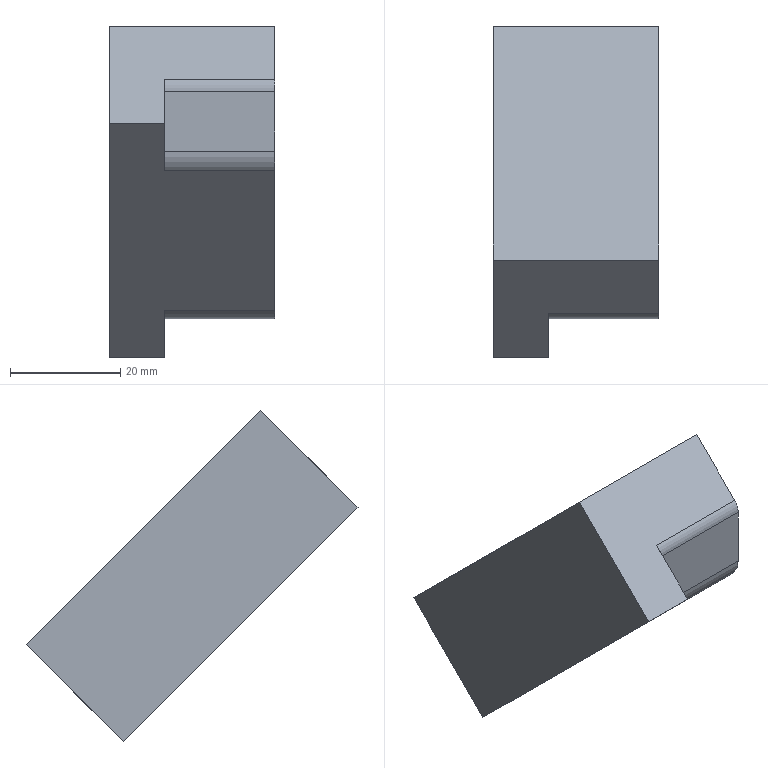Part | NX | features solid 2 | 1 solid | 14 faces | box 30 x 60.104 x 60.104 mm | volume 42971 mm3 | plane 10 | cylinder 4 | commonest cylinder face diameters 6 x2 10 x2
STEP:
#1=CARTESIAN_POINT('',(735.,899.35,-213.579));
#2=VERTEX_POINT('',#1);
#3=CARTESIAN_POINT('',(735.,907.3,-205.629));
#4=VERTEX_POINT('',#3);
#5=CARTESIAN_POINT('',(735.,899.35,-213.579));
#6=DIRECTION('',(0.,0.7071,0.7071));
#7=VECTOR('',#6,1000.);
#8=LINE('',#5,#7);
#9=EDGE_CURVE('',#2,#4,#8,.T.);
#10=ORIENTED_EDGE('',*,*,#9,.F.);
#11=CARTESIAN_POINT('',(735.,907.886,-222.114));
#12=VERTEX_POINT('',#11);
#13=CARTESIAN_POINT('',(735.,899.35,-213.579));
#14=DIRECTION('',(0.,0.7071,-0.7071));
#15=VECTOR('',#14,1000.);
#16=LINE('',#13,#15);
#17=EDGE_CURVE('',#2,#12,#16,.T.);
#18=ORIENTED_EDGE('',*,*,#17,.T.);
#19=CARTESIAN_POINT('',(735.,906.421,-218.579));
#20=VERTEX_POINT('',#19);
#21=CARTESIAN_POINT('',(735.,911.421,-218.579));
#22=DIRECTION('',(-1.,0.,0.));
#23=DIRECTION('',(0.,0.9962,0.08716));
#24=AXIS2_PLACEMENT_3D('',#21,#22,#23);
#25=CIRCLE('',#24,5.);
#26=EDGE_CURVE('',#20,#12,#25,.F.);
#27=ORIENTED_EDGE('',*,*,#26,.F.);
#28=CARTESIAN_POINT('',(735.,906.421,-207.75));
#29=VERTEX_POINT('',#28);
#30=CARTESIAN_POINT('',(735.,906.421,-256.005));
#31=DIRECTION('',(0.,0.,-1.));
#32=VECTOR('',#31,1000.);
#33=LINE('',#30,#32);
#34=EDGE_CURVE('',#29,#20,#33,.T.);
#35=ORIENTED_EDGE('',*,*,#34,.F.);
#36=CARTESIAN_POINT('',(735.,909.421,-207.75));
#37=DIRECTION('',(-1.,0.,0.));
#38=DIRECTION('',(0.,0.9962,0.08716));
#39=AXIS2_PLACEMENT_3D('',#36,#37,#38);
#40=CIRCLE('',#39,3.);
#41=EDGE_CURVE('',#4,#29,#40,.F.);
#42=ORIENTED_EDGE('',*,*,#41,.F.);
#43=EDGE_LOOP('',(#10,#18,#27,#35,#42));
#44=FACE_BOUND('',#43,.T.);
#45=CARTESIAN_POINT('',(735.,941.777,-256.005));
#46=DIRECTION('',(1.,0.,0.));
#47=DIRECTION('',(0.,0.9962,0.08716));
#48=AXIS2_PLACEMENT_3D('',#45,#46,#47);
#49=PLANE('',#48);
#50=ADVANCED_FACE('',(#44),#49,.T.);
#51=CARTESIAN_POINT('',(735.,933.241,-247.47));
#52=VERTEX_POINT('',#51);
#53=CARTESIAN_POINT('',(735.,941.777,-256.005));
#54=VERTEX_POINT('',#53);
#55=CARTESIAN_POINT('',(735.,899.35,-213.579));
#56=DIRECTION('',(0.,0.7071,-0.7071));
#57=VECTOR('',#56,1000.);
#58=LINE('',#55,#57);
#59=EDGE_CURVE('',#52,#54,#58,.T.);
#60=ORIENTED_EDGE('',*,*,#59,.T.);
#61=CARTESIAN_POINT('',(735.,949.726,-248.055));
#62=VERTEX_POINT('',#61);
#63=CARTESIAN_POINT('',(735.,941.777,-256.005));
#64=DIRECTION('',(0.,0.7071,0.7071));
#65=VECTOR('',#64,1000.);
#66=LINE('',#63,#65);
#67=EDGE_CURVE('',#54,#62,#66,.T.);
#68=ORIENTED_EDGE('',*,*,#67,.T.);
#69=CARTESIAN_POINT('',(735.,947.605,-248.934));
#70=VERTEX_POINT('',#69);
#71=CARTESIAN_POINT('',(735.,947.605,-245.934));
#72=DIRECTION('',(-1.,0.,0.));
#73=DIRECTION('',(0.,0.9962,0.08716));
#74=AXIS2_PLACEMENT_3D('',#71,#72,#73);
#75=CIRCLE('',#74,3.);
#76=EDGE_CURVE('',#70,#62,#75,.F.);
#77=ORIENTED_EDGE('',*,*,#76,.F.);
#78=CARTESIAN_POINT('',(735.,936.777,-248.934));
#79=VERTEX_POINT('',#78);
#80=CARTESIAN_POINT('',(735.,941.777,-248.934));
#81=DIRECTION('',(0.,1.,0.));
#82=VECTOR('',#81,1000.);
#83=LINE('',#80,#82);
#84=EDGE_CURVE('',#79,#70,#83,.T.);
#85=ORIENTED_EDGE('',*,*,#84,.F.);
#86=CARTESIAN_POINT('',(735.,936.777,-243.934));
#87=DIRECTION('',(-1.,0.,0.));
#88=DIRECTION('',(0.,0.9962,0.08716));
#89=AXIS2_PLACEMENT_3D('',#86,#87,#88);
#90=CIRCLE('',#89,5.);
#91=EDGE_CURVE('',#52,#79,#90,.F.);
#92=ORIENTED_EDGE('',*,*,#91,.F.);
#93=EDGE_LOOP('',(#60,#68,#77,#85,#92));
#94=FACE_BOUND('',#93,.T.);
#95=CARTESIAN_POINT('',(735.,941.777,-256.005));
#96=DIRECTION('',(1.,0.,0.));
#97=DIRECTION('',(0.,0.9962,0.08716));
#98=AXIS2_PLACEMENT_3D('',#95,#96,#97);
#99=PLANE('',#98);
#100=ADVANCED_FACE('',(#94),#99,.T.);
#101=ORIENTED_EDGE('',*,*,#67,.F.);
#102=CARTESIAN_POINT('',(725.,941.777,-256.005));
#103=VERTEX_POINT('',#102);
#104=CARTESIAN_POINT('',(735.,941.777,-256.005));
#105=DIRECTION('',(-1.,0.,0.));
#106=VECTOR('',#105,1000.);
#107=LINE('',#104,#106);
#108=EDGE_CURVE('',#54,#103,#107,.T.);
#109=ORIENTED_EDGE('',*,*,#108,.T.);
#110=CARTESIAN_POINT('',(725.,959.454,-238.327));
#111=VERTEX_POINT('',#110);
#112=CARTESIAN_POINT('',(725.,941.777,-256.005));
#113=DIRECTION('',(0.,0.7071,0.7071));
#114=VECTOR('',#113,1000.);
#115=LINE('',#112,#114);
#116=EDGE_CURVE('',#103,#111,#115,.T.);
#117=ORIENTED_EDGE('',*,*,#116,.T.);
#118=CARTESIAN_POINT('',(755.,959.454,-238.327));
#119=VERTEX_POINT('',#118);
#120=CARTESIAN_POINT('',(735.,959.454,-238.327));
#121=DIRECTION('',(-1.,0.,0.));
#122=VECTOR('',#121,1000.);
#123=LINE('',#120,#122);
#124=EDGE_CURVE('',#119,#111,#123,.T.);
#125=ORIENTED_EDGE('',*,*,#124,.F.);
#126=CARTESIAN_POINT('',(755.,949.726,-248.055));
#127=VERTEX_POINT('',#126);
#128=CARTESIAN_POINT('',(755.,941.777,-256.005));
#129=DIRECTION('',(0.,0.7071,0.7071));
#130=VECTOR('',#129,1000.);
#131=LINE('',#128,#130);
#132=EDGE_CURVE('',#127,#119,#131,.T.);
#133=ORIENTED_EDGE('',*,*,#132,.F.);
#134=CARTESIAN_POINT('',(755.,949.726,-248.055));
#135=DIRECTION('',(-1.,0.,0.));
#136=VECTOR('',#135,1000.);
#137=LINE('',#134,#136);
#138=EDGE_CURVE('',#62,#127,#137,.F.);
#139=ORIENTED_EDGE('',*,*,#138,.F.);
#140=EDGE_LOOP('',(#101,#109,#117,#125,#133,#139));
#141=FACE_BOUND('',#140,.T.);
#142=CARTESIAN_POINT('',(735.,941.777,-256.005));
#143=DIRECTION('',(0.,0.7071,-0.7071));
#144=DIRECTION('',(0.,0.7071,0.7071));
#145=AXIS2_PLACEMENT_3D('',#142,#143,#144);
#146=PLANE('',#145);
#147=ADVANCED_FACE('',(#141),#146,.T.);
#148=CARTESIAN_POINT('',(725.,917.028,-195.901));
#149=VERTEX_POINT('',#148);
#150=CARTESIAN_POINT('',(725.,917.028,-195.901));
#151=DIRECTION('',(0.,0.7071,-0.7071));
#152=VECTOR('',#151,1000.);
#153=LINE('',#150,#152);
#154=EDGE_CURVE('',#149,#111,#153,.T.);
#155=ORIENTED_EDGE('',*,*,#154,.F.);
#156=CARTESIAN_POINT('',(755.,917.028,-195.901));
#157=VERTEX_POINT('',#156);
#158=CARTESIAN_POINT('',(735.,917.028,-195.901));
#159=DIRECTION('',(-1.,0.,0.));
#160=VECTOR('',#159,1000.);
#161=LINE('',#158,#160);
#162=EDGE_CURVE('',#157,#149,#161,.T.);
#163=ORIENTED_EDGE('',*,*,#162,.F.);
#164=CARTESIAN_POINT('',(755.,917.028,-195.901));
#165=DIRECTION('',(0.,0.7071,-0.7071));
#166=VECTOR('',#165,1000.);
#167=LINE('',#164,#166);
#168=EDGE_CURVE('',#157,#119,#167,.T.);
#169=ORIENTED_EDGE('',*,*,#168,.T.);
#170=ORIENTED_EDGE('',*,*,#124,.T.);
#171=EDGE_LOOP('',(#155,#163,#169,#170));
#172=FACE_BOUND('',#171,.T.);
#173=CARTESIAN_POINT('',(735.,917.028,-195.901));
#174=DIRECTION('',(0.,-0.7071,-0.7071));
#175=DIRECTION('',(0.,0.7071,-0.7071));
#176=AXIS2_PLACEMENT_3D('',#173,#174,#175);
#177=PLANE('',#176);
#178=ADVANCED_FACE('',(#172),#177,.F.);
#179=CARTESIAN_POINT('',(755.,907.3,-205.629));
#180=VERTEX_POINT('',#179);
#181=CARTESIAN_POINT('',(755.,899.35,-213.579));
#182=DIRECTION('',(0.,0.7071,0.7071));
#183=VECTOR('',#182,1000.);
#184=LINE('',#181,#183);
#185=EDGE_CURVE('',#180,#157,#184,.T.);
#186=ORIENTED_EDGE('',*,*,#185,.T.);
#187=ORIENTED_EDGE('',*,*,#162,.T.);
#188=CARTESIAN_POINT('',(725.,899.35,-213.579));
#189=VERTEX_POINT('',#188);
#190=CARTESIAN_POINT('',(725.,899.35,-213.579));
#191=DIRECTION('',(0.,0.7071,0.7071));
#192=VECTOR('',#191,1000.);
#193=LINE('',#190,#192);
#194=EDGE_CURVE('',#189,#149,#193,.T.);
#195=ORIENTED_EDGE('',*,*,#194,.F.);
#196=CARTESIAN_POINT('',(735.,899.35,-213.579));
#197=DIRECTION('',(-1.,0.,0.));
#198=VECTOR('',#197,1000.);
#199=LINE('',#196,#198);
#200=EDGE_CURVE('',#2,#189,#199,.T.);
#201=ORIENTED_EDGE('',*,*,#200,.F.);
#202=ORIENTED_EDGE('',*,*,#9,.T.);
#203=CARTESIAN_POINT('',(735.,907.3,-205.629));
#204=DIRECTION('',(-1.,0.,0.));
#205=VECTOR('',#204,1000.);
#206=LINE('',#203,#205);
#207=EDGE_CURVE('',#180,#4,#206,.T.);
#208=ORIENTED_EDGE('',*,*,#207,.F.);
#209=EDGE_LOOP('',(#186,#187,#195,#201,#202,#208));
#210=FACE_BOUND('',#209,.T.);
#211=CARTESIAN_POINT('',(735.,899.35,-213.579));
#212=DIRECTION('',(0.,0.7071,-0.7071));
#213=DIRECTION('',(0.,0.7071,0.7071));
#214=AXIS2_PLACEMENT_3D('',#211,#212,#213);
#215=PLANE('',#214);
#216=ADVANCED_FACE('',(#210),#215,.F.);
#217=CARTESIAN_POINT('',(755.,907.886,-222.114));
#218=VERTEX_POINT('',#217);
#219=CARTESIAN_POINT('',(755.,933.241,-247.47));
#220=VERTEX_POINT('',#219);
#221=CARTESIAN_POINT('',(755.,899.35,-213.579));
#222=DIRECTION('',(0.,0.7071,-0.7071));
#223=VECTOR('',#222,1000.);
#224=LINE('',#221,#223);
#225=EDGE_CURVE('',#218,#220,#224,.T.);
#226=ORIENTED_EDGE('',*,*,#225,.F.);
#227=CARTESIAN_POINT('',(755.,907.886,-222.114));
#228=DIRECTION('',(-1.,0.,0.));
#229=VECTOR('',#228,1000.);
#230=LINE('',#227,#229);
#231=EDGE_CURVE('',#12,#218,#230,.F.);
#232=ORIENTED_EDGE('',*,*,#231,.F.);
#233=ORIENTED_EDGE('',*,*,#17,.F.);
#234=ORIENTED_EDGE('',*,*,#200,.T.);
#235=CARTESIAN_POINT('',(725.,899.35,-213.579));
#236=DIRECTION('',(0.,0.7071,-0.7071));
#237=VECTOR('',#236,1000.);
#238=LINE('',#235,#237);
#239=EDGE_CURVE('',#189,#103,#238,.T.);
#240=ORIENTED_EDGE('',*,*,#239,.T.);
#241=ORIENTED_EDGE('',*,*,#108,.F.);
#242=ORIENTED_EDGE('',*,*,#59,.F.);
#243=CARTESIAN_POINT('',(735.,933.241,-247.47));
#244=DIRECTION('',(-1.,0.,0.));
#245=VECTOR('',#244,1000.);
#246=LINE('',#243,#245);
#247=EDGE_CURVE('',#220,#52,#246,.T.);
#248=ORIENTED_EDGE('',*,*,#247,.F.);
#249=EDGE_LOOP('',(#226,#232,#233,#234,#240,#241,#242,#248));
#250=FACE_BOUND('',#249,.T.);
#251=CARTESIAN_POINT('',(735.,899.35,-213.579));
#252=DIRECTION('',(0.,-0.7071,-0.7071));
#253=DIRECTION('',(0.,0.7071,-0.7071));
#254=AXIS2_PLACEMENT_3D('',#251,#252,#253);
#255=PLANE('',#254);
#256=ADVANCED_FACE('',(#250),#255,.T.);
#257=ORIENTED_EDGE('',*,*,#154,.T.);
#258=ORIENTED_EDGE('',*,*,#116,.F.);
#259=ORIENTED_EDGE('',*,*,#239,.F.);
#260=ORIENTED_EDGE('',*,*,#194,.T.);
#261=EDGE_LOOP('',(#257,#258,#259,#260));
#262=FACE_BOUND('',#261,.T.);
#263=CARTESIAN_POINT('',(725.,941.777,-256.005));
#264=DIRECTION('',(1.,0.,0.));
#265=DIRECTION('',(0.,0.9962,0.08716));
#266=AXIS2_PLACEMENT_3D('',#263,#264,#265);
#267=PLANE('',#266);
#268=ADVANCED_FACE('',(#262),#267,.F.);
#269=CARTESIAN_POINT('',(755.,906.421,-218.579));
#270=VERTEX_POINT('',#269);
#271=CARTESIAN_POINT('',(755.,906.421,-207.75));
#272=VERTEX_POINT('',#271);
#273=CARTESIAN_POINT('',(755.,906.421,-220.65));
#274=DIRECTION('',(0.,0.,1.));
#275=VECTOR('',#274,1000.);
#276=LINE('',#273,#275);
#277=EDGE_CURVE('',#270,#272,#276,.T.);
#278=ORIENTED_EDGE('',*,*,#277,.T.);
#279=CARTESIAN_POINT('',(755.,906.421,-207.75));
#280=DIRECTION('',(-1.,0.,0.));
#281=VECTOR('',#280,1000.);
#282=LINE('',#279,#281);
#283=EDGE_CURVE('',#29,#272,#282,.F.);
#284=ORIENTED_EDGE('',*,*,#283,.F.);
#285=ORIENTED_EDGE('',*,*,#34,.T.);
#286=CARTESIAN_POINT('',(735.,906.421,-218.579));
#287=DIRECTION('',(-1.,0.,0.));
#288=VECTOR('',#287,1000.);
#289=LINE('',#286,#288);
#290=EDGE_CURVE('',#270,#20,#289,.T.);
#291=ORIENTED_EDGE('',*,*,#290,.F.);
#292=EDGE_LOOP('',(#278,#284,#285,#291));
#293=FACE_BOUND('',#292,.T.);
#294=CARTESIAN_POINT('',(755.,906.421,-220.65));
#295=DIRECTION('',(0.,1.,0.));
#296=DIRECTION('',(0.,0.,1.));
#297=AXIS2_PLACEMENT_3D('',#294,#295,#296);
#298=PLANE('',#297);
#299=ADVANCED_FACE('',(#293),#298,.F.);
#300=ORIENTED_EDGE('',*,*,#84,.T.);
#301=CARTESIAN_POINT('',(755.,947.605,-248.934));
#302=VERTEX_POINT('',#301);
#303=CARTESIAN_POINT('',(735.,947.605,-248.934));
#304=DIRECTION('',(-1.,0.,0.));
#305=VECTOR('',#304,1000.);
#306=LINE('',#303,#305);
#307=EDGE_CURVE('',#302,#70,#306,.T.);
#308=ORIENTED_EDGE('',*,*,#307,.F.);
#309=CARTESIAN_POINT('',(755.,936.777,-248.934));
#310=VERTEX_POINT('',#309);
#311=CARTESIAN_POINT('',(755.,948.848,-248.934));
#312=DIRECTION('',(0.,-1.,0.));
#313=VECTOR('',#312,1000.);
#314=LINE('',#311,#313);
#315=EDGE_CURVE('',#302,#310,#314,.T.);
#316=ORIENTED_EDGE('',*,*,#315,.T.);
#317=CARTESIAN_POINT('',(755.,936.777,-248.934));
#318=DIRECTION('',(-1.,0.,0.));
#319=VECTOR('',#318,1000.);
#320=LINE('',#317,#319);
#321=EDGE_CURVE('',#79,#310,#320,.F.);
#322=ORIENTED_EDGE('',*,*,#321,.F.);
#323=EDGE_LOOP('',(#300,#308,#316,#322));
#324=FACE_BOUND('',#323,.T.);
#325=CARTESIAN_POINT('',(755.,948.848,-248.934));
#326=DIRECTION('',(0.,0.,1.));
#327=DIRECTION('',(0.,-1.,0.));
#328=AXIS2_PLACEMENT_3D('',#325,#326,#327);
#329=PLANE('',#328);
#330=ADVANCED_FACE('',(#324),#329,.F.);
#331=ORIENTED_EDGE('',*,*,#315,.F.);
#332=CARTESIAN_POINT('',(755.,947.605,-245.934));
#333=DIRECTION('',(1.,0.,0.));
#334=DIRECTION('',(0.,-0.9962,-0.08716));
#335=AXIS2_PLACEMENT_3D('',#332,#333,#334);
#336=CIRCLE('',#335,3.);
#337=EDGE_CURVE('',#127,#302,#336,.F.);
#338=ORIENTED_EDGE('',*,*,#337,.F.);
#339=ORIENTED_EDGE('',*,*,#132,.T.);
#340=ORIENTED_EDGE('',*,*,#168,.F.);
#341=ORIENTED_EDGE('',*,*,#185,.F.);
#342=CARTESIAN_POINT('',(755.,909.421,-207.75));
#343=DIRECTION('',(1.,0.,0.));
#344=DIRECTION('',(0.,-0.9962,-0.08716));
#345=AXIS2_PLACEMENT_3D('',#342,#343,#344);
#346=CIRCLE('',#345,3.);
#347=EDGE_CURVE('',#272,#180,#346,.F.);
#348=ORIENTED_EDGE('',*,*,#347,.F.);
#349=ORIENTED_EDGE('',*,*,#277,.F.);
#350=CARTESIAN_POINT('',(755.,911.421,-218.579));
#351=DIRECTION('',(1.,0.,0.));
#352=DIRECTION('',(0.,-0.9962,-0.08716));
#353=AXIS2_PLACEMENT_3D('',#350,#351,#352);
#354=CIRCLE('',#353,5.);
#355=EDGE_CURVE('',#218,#270,#354,.F.);
#356=ORIENTED_EDGE('',*,*,#355,.F.);
#357=ORIENTED_EDGE('',*,*,#225,.T.);
#358=CARTESIAN_POINT('',(755.,936.777,-243.934));
#359=DIRECTION('',(1.,0.,0.));
#360=DIRECTION('',(0.,-0.9962,-0.08716));
#361=AXIS2_PLACEMENT_3D('',#358,#359,#360);
#362=CIRCLE('',#361,5.);
#363=EDGE_CURVE('',#310,#220,#362,.F.);
#364=ORIENTED_EDGE('',*,*,#363,.F.);
#365=EDGE_LOOP('',(#331,#338,#339,#340,#341,#348,#349,#356,#357,#364));
#366=FACE_BOUND('',#365,.T.);
#367=CARTESIAN_POINT('',(755.,918.796,-224.775));
#368=DIRECTION('',(-1.,0.,0.));
#369=DIRECTION('',(0.,-0.9962,-0.08716));
#370=AXIS2_PLACEMENT_3D('',#367,#368,#369);
#371=PLANE('',#370);
#372=ADVANCED_FACE('',(#366),#371,.F.);
#373=ORIENTED_EDGE('',*,*,#347,.T.);
#374=ORIENTED_EDGE('',*,*,#207,.T.);
#375=ORIENTED_EDGE('',*,*,#41,.T.);
#376=ORIENTED_EDGE('',*,*,#283,.T.);
#377=EDGE_LOOP('',(#373,#374,#375,#376));
#378=FACE_BOUND('',#377,.T.);
#379=CARTESIAN_POINT('',(735.,909.421,-207.75));
#380=DIRECTION('',(-1.,0.,0.));
#381=DIRECTION('',(0.,-0.9962,-0.08716));
#382=AXIS2_PLACEMENT_3D('',#379,#380,#381);
#383=CYLINDRICAL_SURFACE('',#382,3.);
#384=ADVANCED_FACE('',(#378),#383,.T.);
#385=ORIENTED_EDGE('',*,*,#337,.T.);
#386=ORIENTED_EDGE('',*,*,#307,.T.);
#387=ORIENTED_EDGE('',*,*,#76,.T.);
#388=ORIENTED_EDGE('',*,*,#138,.T.);
#389=EDGE_LOOP('',(#385,#386,#387,#388));
#390=FACE_BOUND('',#389,.T.);
#391=CARTESIAN_POINT('',(755.,947.605,-245.934));
#392=DIRECTION('',(1.,0.,0.));
#393=DIRECTION('',(0.,0.9962,0.08716));
#394=AXIS2_PLACEMENT_3D('',#391,#392,#393);
#395=CYLINDRICAL_SURFACE('',#394,3.);
#396=ADVANCED_FACE('',(#390),#395,.T.);
#397=ORIENTED_EDGE('',*,*,#363,.T.);
#398=ORIENTED_EDGE('',*,*,#247,.T.);
#399=ORIENTED_EDGE('',*,*,#91,.T.);
#400=ORIENTED_EDGE('',*,*,#321,.T.);
#401=EDGE_LOOP('',(#397,#398,#399,#400));
#402=FACE_BOUND('',#401,.T.);
#403=CARTESIAN_POINT('',(735.,936.777,-243.934));
#404=DIRECTION('',(1.,0.,0.));
#405=DIRECTION('',(0.,0.9962,0.08716));
#406=AXIS2_PLACEMENT_3D('',#403,#404,#405);
#407=CYLINDRICAL_SURFACE('',#406,5.);
#408=ADVANCED_FACE('',(#402),#407,.T.);
#409=ORIENTED_EDGE('',*,*,#355,.T.);
#410=ORIENTED_EDGE('',*,*,#290,.T.);
#411=ORIENTED_EDGE('',*,*,#26,.T.);
#412=ORIENTED_EDGE('',*,*,#231,.T.);
#413=EDGE_LOOP('',(#409,#410,#411,#412));
#414=FACE_BOUND('',#413,.T.);
#415=CARTESIAN_POINT('',(755.,911.421,-218.579));
#416=DIRECTION('',(1.,0.,0.));
#417=DIRECTION('',(0.,0.9962,0.08716));
#418=AXIS2_PLACEMENT_3D('',#415,#416,#417);
#419=CYLINDRICAL_SURFACE('',#418,5.);
#420=ADVANCED_FACE('',(#414),#419,.T.);
#421=CLOSED_SHELL('',(#50,#100,#147,#178,#216,#256,#268,#299,#330,#372,#384,#396,#408,#420));
#422=MANIFOLD_SOLID_BREP('',#421);
#423=(LENGTH_UNIT()NAMED_UNIT(*)SI_UNIT(.MILLI.,.METRE.));
#424=UNCERTAINTY_MEASURE_WITH_UNIT(LENGTH_MEASURE(0.00001),#423,'','');
#425=(NAMED_UNIT(*)PLANE_ANGLE_UNIT()SI_UNIT($,.RADIAN.));
#426=(NAMED_UNIT(*)SI_UNIT($,.STERADIAN.)SOLID_ANGLE_UNIT());
#427=(GEOMETRIC_REPRESENTATION_CONTEXT(3)GLOBAL_UNCERTAINTY_ASSIGNED_CONTEXT((#424))GLOBAL_UNIT_ASSIGNED_CONTEXT((#423,#425,#426))REPRESENTATION_CONTEXT('',''));
#428=ADVANCED_BREP_SHAPE_REPRESENTATION('',(#422),#427);